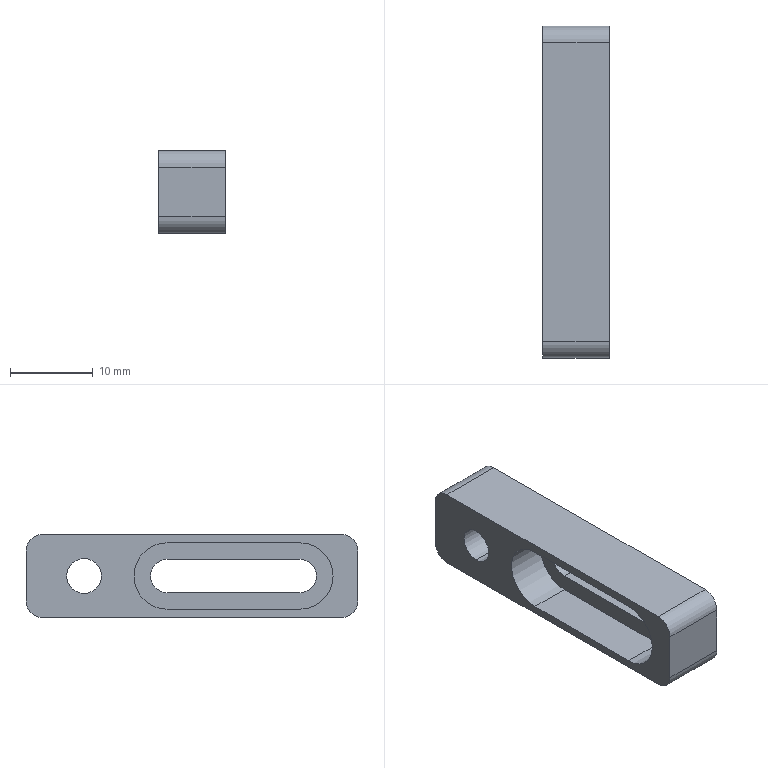Part | SolidWorks | features Fillet 2, ICE 2, Extrusion 1, HoleWzd 1 | 1 solid | 23 faces | box 8 x 40 x 10 mm | volume 1941 mm3 | cylinder 12 | plane 11 | commonest cylinder face diameters 4 x7 8 x3 4.2 x2
STEP:
#1=CARTESIAN_POINT('',(-4.756,11.524,5.));
#2=VERTEX_POINT('',#1);
#3=CARTESIAN_POINT('',(-4.756,15.524,9.));
#4=VERTEX_POINT('',#3);
#5=CARTESIAN_POINT('',(-4.756,15.524,5.));
#6=DIRECTION('',(-1.,0.,0.));
#7=DIRECTION('',(0.,-1.,0.));
#8=AXIS2_PLACEMENT_3D('',#5,#6,#7);
#9=CIRCLE('',#8,4.);
#10=EDGE_CURVE('',#2,#4,#9,.T.);
#11=ORIENTED_EDGE('',*,*,#10,.F.);
#12=CARTESIAN_POINT('',(-9.756,11.524,5.));
#13=VERTEX_POINT('',#12);
#14=CARTESIAN_POINT('',(-4.756,11.524,5.));
#15=DIRECTION('',(-1.,0.,0.));
#16=VECTOR('',#15,1000.);
#17=LINE('',#14,#16);
#18=EDGE_CURVE('',#2,#13,#17,.T.);
#19=ORIENTED_EDGE('',*,*,#18,.T.);
#20=CARTESIAN_POINT('',(-9.756,15.524,9.));
#21=VERTEX_POINT('',#20);
#22=CARTESIAN_POINT('',(-9.756,15.524,5.));
#23=DIRECTION('',(-1.,0.,0.));
#24=DIRECTION('',(0.,-1.,0.));
#25=AXIS2_PLACEMENT_3D('',#22,#23,#24);
#26=CIRCLE('',#25,4.);
#27=EDGE_CURVE('',#13,#21,#26,.T.);
#28=ORIENTED_EDGE('',*,*,#27,.T.);
#29=CARTESIAN_POINT('',(-4.756,15.524,9.));
#30=DIRECTION('',(-1.,0.,0.));
#31=VECTOR('',#30,1000.);
#32=LINE('',#29,#31);
#33=EDGE_CURVE('',#4,#21,#32,.T.);
#34=ORIENTED_EDGE('',*,*,#33,.F.);
#35=EDGE_LOOP('',(#11,#19,#28,#34));
#36=FACE_OUTER_BOUND('',#35,.T.);
#37=CARTESIAN_POINT('',(-4.756,15.524,5.));
#38=DIRECTION('',(-1.,0.,0.));
#39=DIRECTION('',(0.,-1.,0.));
#40=AXIS2_PLACEMENT_3D('',#37,#38,#39);
#41=CYLINDRICAL_SURFACE('',#40,4.);
#42=ADVANCED_FACE('',(#36),#41,.F.);
#43=CARTESIAN_POINT('',(-9.756,41.524,7.1));
#44=VERTEX_POINT('',#43);
#45=CARTESIAN_POINT('',(-9.756,41.524,2.9));
#46=VERTEX_POINT('',#45);
#47=CARTESIAN_POINT('',(-9.756,41.524,5.));
#48=DIRECTION('',(1.,0.,0.));
#49=DIRECTION('',(0.,1.,0.));
#50=AXIS2_PLACEMENT_3D('',#47,#48,#49);
#51=CIRCLE('',#50,2.1);
#52=EDGE_CURVE('',#44,#46,#51,.T.);
#53=ORIENTED_EDGE('',*,*,#52,.F.);
#54=CARTESIAN_POINT('',(-1.756,41.524,7.1));
#55=VERTEX_POINT('',#54);
#56=CARTESIAN_POINT('',(-1.756,41.524,7.1));
#57=DIRECTION('',(1.,0.,0.));
#58=VECTOR('',#57,1000.);
#59=LINE('',#56,#58);
#60=EDGE_CURVE('',#44,#55,#59,.T.);
#61=ORIENTED_EDGE('',*,*,#60,.T.);
#62=CARTESIAN_POINT('',(-1.756,41.524,2.9));
#63=VERTEX_POINT('',#62);
#64=CARTESIAN_POINT('',(-1.756,41.524,5.));
#65=DIRECTION('',(1.,0.,0.));
#66=DIRECTION('',(0.,0.,-1.));
#67=AXIS2_PLACEMENT_3D('',#64,#65,#66);
#68=CIRCLE('',#67,2.1);
#69=EDGE_CURVE('',#55,#63,#68,.T.);
#70=ORIENTED_EDGE('',*,*,#69,.T.);
#71=CARTESIAN_POINT('',(-1.756,41.524,2.9));
#72=DIRECTION('',(1.,0.,0.));
#73=VECTOR('',#72,1000.);
#74=LINE('',#71,#73);
#75=EDGE_CURVE('',#46,#63,#74,.T.);
#76=ORIENTED_EDGE('',*,*,#75,.F.);
#77=EDGE_LOOP('',(#53,#61,#70,#76));
#78=FACE_OUTER_BOUND('',#77,.T.);
#79=CARTESIAN_POINT('',(-1.756,41.524,5.));
#80=DIRECTION('',(1.,0.,0.));
#81=DIRECTION('',(0.,0.,-1.));
#82=AXIS2_PLACEMENT_3D('',#79,#80,#81);
#83=CYLINDRICAL_SURFACE('',#82,2.1);
#84=ADVANCED_FACE('',(#78),#83,.F.);
#85=CARTESIAN_POINT('',(-1.756,13.524,5.));
#86=VERTEX_POINT('',#85);
#87=CARTESIAN_POINT('',(-1.756,15.524,7.));
#88=VERTEX_POINT('',#87);
#89=CARTESIAN_POINT('',(-1.756,15.524,5.));
#90=DIRECTION('',(-1.,0.,0.));
#91=DIRECTION('',(0.,-1.,0.));
#92=AXIS2_PLACEMENT_3D('',#89,#90,#91);
#93=CIRCLE('',#92,2.);
#94=EDGE_CURVE('',#86,#88,#93,.T.);
#95=ORIENTED_EDGE('',*,*,#94,.F.);
#96=CARTESIAN_POINT('',(-4.756,13.524,5.));
#97=VERTEX_POINT('',#96);
#98=CARTESIAN_POINT('',(-1.756,13.524,5.));
#99=DIRECTION('',(-1.,0.,0.));
#100=VECTOR('',#99,1000.);
#101=LINE('',#98,#100);
#102=EDGE_CURVE('',#86,#97,#101,.T.);
#103=ORIENTED_EDGE('',*,*,#102,.T.);
#104=CARTESIAN_POINT('',(-4.756,15.524,7.));
#105=VERTEX_POINT('',#104);
#106=CARTESIAN_POINT('',(-4.756,15.524,5.));
#107=DIRECTION('',(1.,0.,0.));
#108=DIRECTION('',(0.,-1.,0.));
#109=AXIS2_PLACEMENT_3D('',#106,#107,#108);
#110=CIRCLE('',#109,2.);
#111=EDGE_CURVE('',#105,#97,#110,.T.);
#112=ORIENTED_EDGE('',*,*,#111,.F.);
#113=CARTESIAN_POINT('',(-1.756,15.524,7.));
#114=DIRECTION('',(-1.,0.,0.));
#115=VECTOR('',#114,1000.);
#116=LINE('',#113,#115);
#117=EDGE_CURVE('',#88,#105,#116,.T.);
#118=ORIENTED_EDGE('',*,*,#117,.F.);
#119=EDGE_LOOP('',(#95,#103,#112,#118));
#120=FACE_OUTER_BOUND('',#119,.T.);
#121=CARTESIAN_POINT('',(-1.756,15.524,5.));
#122=DIRECTION('',(-1.,0.,0.));
#123=DIRECTION('',(0.,-1.,0.));
#124=AXIS2_PLACEMENT_3D('',#121,#122,#123);
#125=CYLINDRICAL_SURFACE('',#124,2.);
#126=ADVANCED_FACE('',(#120),#125,.F.);
#127=ORIENTED_EDGE('',*,*,#102,.F.);
#128=CARTESIAN_POINT('',(-1.756,15.524,3.));
#129=VERTEX_POINT('',#128);
#130=CARTESIAN_POINT('',(-1.756,15.524,5.));
#131=DIRECTION('',(-1.,0.,0.));
#132=DIRECTION('',(0.,-1.,0.));
#133=AXIS2_PLACEMENT_3D('',#130,#131,#132);
#134=CIRCLE('',#133,2.);
#135=EDGE_CURVE('',#129,#86,#134,.T.);
#136=ORIENTED_EDGE('',*,*,#135,.F.);
#137=CARTESIAN_POINT('',(-4.756,15.524,3.));
#138=VERTEX_POINT('',#137);
#139=CARTESIAN_POINT('',(-1.756,15.524,3.));
#140=DIRECTION('',(-1.,0.,0.));
#141=VECTOR('',#140,1000.);
#142=LINE('',#139,#141);
#143=EDGE_CURVE('',#129,#138,#142,.T.);
#144=ORIENTED_EDGE('',*,*,#143,.T.);
#145=CARTESIAN_POINT('',(-4.756,15.524,5.));
#146=DIRECTION('',(1.,0.,0.));
#147=DIRECTION('',(0.,-1.,0.));
#148=AXIS2_PLACEMENT_3D('',#145,#146,#147);
#149=CIRCLE('',#148,2.);
#150=EDGE_CURVE('',#97,#138,#149,.T.);
#151=ORIENTED_EDGE('',*,*,#150,.F.);
#152=EDGE_LOOP('',(#127,#136,#144,#151));
#153=FACE_OUTER_BOUND('',#152,.T.);
#154=CARTESIAN_POINT('',(-1.756,15.524,5.));
#155=DIRECTION('',(-1.,0.,0.));
#156=DIRECTION('',(0.,-1.,0.));
#157=AXIS2_PLACEMENT_3D('',#154,#155,#156);
#158=CYLINDRICAL_SURFACE('',#157,2.);
#159=ADVANCED_FACE('',(#153),#158,.F.);
#160=CARTESIAN_POINT('',(-4.756,31.524,3.));
#161=VERTEX_POINT('',#160);
#162=CARTESIAN_POINT('',(-4.756,15.524,3.));
#163=DIRECTION('',(0.,1.,0.));
#164=VECTOR('',#163,1000.);
#165=LINE('',#162,#164);
#166=EDGE_CURVE('',#138,#161,#165,.T.);
#167=ORIENTED_EDGE('',*,*,#166,.F.);
#168=ORIENTED_EDGE('',*,*,#143,.F.);
#169=CARTESIAN_POINT('',(-1.756,31.524,3.));
#170=VERTEX_POINT('',#169);
#171=CARTESIAN_POINT('',(-1.756,15.524,3.));
#172=DIRECTION('',(0.,-1.,0.));
#173=VECTOR('',#172,1000.);
#174=LINE('',#171,#173);
#175=EDGE_CURVE('',#170,#129,#174,.T.);
#176=ORIENTED_EDGE('',*,*,#175,.F.);
#177=CARTESIAN_POINT('',(-1.756,31.524,3.));
#178=DIRECTION('',(-1.,0.,0.));
#179=VECTOR('',#178,1000.);
#180=LINE('',#177,#179);
#181=EDGE_CURVE('',#170,#161,#180,.T.);
#182=ORIENTED_EDGE('',*,*,#181,.T.);
#183=EDGE_LOOP('',(#167,#168,#176,#182));
#184=FACE_OUTER_BOUND('',#183,.T.);
#185=CARTESIAN_POINT('',(-1.756,15.524,3.));
#186=DIRECTION('',(0.,0.,-1.));
#187=DIRECTION('',(-1.,0.,0.));
#188=AXIS2_PLACEMENT_3D('',#185,#186,#187);
#189=PLANE('',#188);
#190=ADVANCED_FACE('',(#184),#189,.F.);
#191=CARTESIAN_POINT('',(-4.756,31.524,7.));
#192=VERTEX_POINT('',#191);
#193=CARTESIAN_POINT('',(-4.756,31.524,5.));
#194=DIRECTION('',(1.,0.,0.));
#195=DIRECTION('',(0.,-1.,0.));
#196=AXIS2_PLACEMENT_3D('',#193,#194,#195);
#197=CIRCLE('',#196,2.);
#198=EDGE_CURVE('',#161,#192,#197,.T.);
#199=ORIENTED_EDGE('',*,*,#198,.F.);
#200=ORIENTED_EDGE('',*,*,#181,.F.);
#201=CARTESIAN_POINT('',(-1.756,31.524,7.));
#202=VERTEX_POINT('',#201);
#203=CARTESIAN_POINT('',(-1.756,31.524,5.));
#204=DIRECTION('',(-1.,0.,0.));
#205=DIRECTION('',(0.,-1.,0.));
#206=AXIS2_PLACEMENT_3D('',#203,#204,#205);
#207=CIRCLE('',#206,2.);
#208=EDGE_CURVE('',#202,#170,#207,.T.);
#209=ORIENTED_EDGE('',*,*,#208,.F.);
#210=CARTESIAN_POINT('',(-1.756,31.524,7.));
#211=DIRECTION('',(-1.,0.,0.));
#212=VECTOR('',#211,1000.);
#213=LINE('',#210,#212);
#214=EDGE_CURVE('',#202,#192,#213,.T.);
#215=ORIENTED_EDGE('',*,*,#214,.T.);
#216=EDGE_LOOP('',(#199,#200,#209,#215));
#217=FACE_OUTER_BOUND('',#216,.T.);
#218=CARTESIAN_POINT('',(-1.756,31.524,5.));
#219=DIRECTION('',(-1.,0.,0.));
#220=DIRECTION('',(0.,-1.,0.));
#221=AXIS2_PLACEMENT_3D('',#218,#219,#220);
#222=CYLINDRICAL_SURFACE('',#221,2.);
#223=ADVANCED_FACE('',(#217),#222,.F.);
#224=CARTESIAN_POINT('',(-4.756,15.524,7.));
#225=DIRECTION('',(0.,-1.,0.));
#226=VECTOR('',#225,1000.);
#227=LINE('',#224,#226);
#228=EDGE_CURVE('',#192,#105,#227,.T.);
#229=ORIENTED_EDGE('',*,*,#228,.F.);
#230=ORIENTED_EDGE('',*,*,#214,.F.);
#231=CARTESIAN_POINT('',(-1.756,15.524,7.));
#232=DIRECTION('',(0.,1.,0.));
#233=VECTOR('',#232,1000.);
#234=LINE('',#231,#233);
#235=EDGE_CURVE('',#88,#202,#234,.T.);
#236=ORIENTED_EDGE('',*,*,#235,.F.);
#237=ORIENTED_EDGE('',*,*,#117,.T.);
#238=EDGE_LOOP('',(#229,#230,#236,#237));
#239=FACE_OUTER_BOUND('',#238,.T.);
#240=CARTESIAN_POINT('',(-1.756,15.524,7.));
#241=DIRECTION('',(0.,0.,1.));
#242=DIRECTION('',(1.,0.,0.));
#243=AXIS2_PLACEMENT_3D('',#240,#241,#242);
#244=PLANE('',#243);
#245=ADVANCED_FACE('',(#239),#244,.F.);
#246=CARTESIAN_POINT('',(-9.756,8.524,8.));
#247=VERTEX_POINT('',#246);
#248=CARTESIAN_POINT('',(-9.756,8.524,2.));
#249=VERTEX_POINT('',#248);
#250=CARTESIAN_POINT('',(-9.756,8.524,10.));
#251=DIRECTION('',(0.,0.,-1.));
#252=VECTOR('',#251,1000.);
#253=LINE('',#250,#252);
#254=EDGE_CURVE('',#247,#249,#253,.T.);
#255=ORIENTED_EDGE('',*,*,#254,.T.);
#256=CARTESIAN_POINT('',(-1.756,8.524,2.));
#257=VERTEX_POINT('',#256);
#258=CARTESIAN_POINT('',(-1.756,8.524,2.));
#259=DIRECTION('',(1.,0.,0.));
#260=VECTOR('',#259,1000.);
#261=LINE('',#258,#260);
#262=EDGE_CURVE('',#249,#257,#261,.T.);
#263=ORIENTED_EDGE('',*,*,#262,.T.);
#264=CARTESIAN_POINT('',(-1.756,8.524,8.));
#265=VERTEX_POINT('',#264);
#266=CARTESIAN_POINT('',(-1.756,8.524,10.));
#267=DIRECTION('',(0.,0.,-1.));
#268=VECTOR('',#267,1000.);
#269=LINE('',#266,#268);
#270=EDGE_CURVE('',#265,#257,#269,.T.);
#271=ORIENTED_EDGE('',*,*,#270,.F.);
#272=CARTESIAN_POINT('',(-9.756,8.524,8.));
#273=DIRECTION('',(-1.,0.,0.));
#274=VECTOR('',#273,1000.);
#275=LINE('',#272,#274);
#276=EDGE_CURVE('',#265,#247,#275,.T.);
#277=ORIENTED_EDGE('',*,*,#276,.T.);
#278=EDGE_LOOP('',(#255,#263,#271,#277));
#279=FACE_OUTER_BOUND('',#278,.T.);
#280=CARTESIAN_POINT('',(-1.756,8.524,10.));
#281=DIRECTION('',(0.,1.,0.));
#282=DIRECTION('',(-1.,0.,0.));
#283=AXIS2_PLACEMENT_3D('',#280,#281,#282);
#284=PLANE('',#283);
#285=ADVANCED_FACE('',(#279),#284,.F.);
#286=ORIENTED_EDGE('',*,*,#175,.T.);
#287=ORIENTED_EDGE('',*,*,#135,.T.);
#288=ORIENTED_EDGE('',*,*,#94,.T.);
#289=ORIENTED_EDGE('',*,*,#235,.T.);
#290=ORIENTED_EDGE('',*,*,#208,.T.);
#291=EDGE_LOOP('',(#286,#287,#288,#289,#290));
#292=FACE_BOUND('',#291,.T.);
#293=CARTESIAN_POINT('',(-1.756,41.524,5.));
#294=DIRECTION('',(1.,0.,0.));
#295=DIRECTION('',(0.,0.,-1.));
#296=AXIS2_PLACEMENT_3D('',#293,#294,#295);
#297=CIRCLE('',#296,2.1);
#298=EDGE_CURVE('',#63,#55,#297,.T.);
#299=ORIENTED_EDGE('',*,*,#298,.F.);
#300=ORIENTED_EDGE('',*,*,#69,.F.);
#301=EDGE_LOOP('',(#299,#300));
#302=FACE_BOUND('',#301,.T.);
#303=ORIENTED_EDGE('',*,*,#270,.T.);
#304=CARTESIAN_POINT('',(-1.756,10.524,0.));
#305=VERTEX_POINT('',#304);
#306=CARTESIAN_POINT('',(-1.756,10.524,2.));
#307=DIRECTION('',(1.,0.,0.));
#308=DIRECTION('',(0.,-1.,0.));
#309=AXIS2_PLACEMENT_3D('',#306,#307,#308);
#310=CIRCLE('',#309,2.);
#311=EDGE_CURVE('',#257,#305,#310,.T.);
#312=ORIENTED_EDGE('',*,*,#311,.T.);
#313=CARTESIAN_POINT('',(-1.756,46.524,0.));
#314=VERTEX_POINT('',#313);
#315=CARTESIAN_POINT('',(-1.756,48.524,0.));
#316=DIRECTION('',(0.,1.,0.));
#317=VECTOR('',#316,1000.);
#318=LINE('',#315,#317);
#319=EDGE_CURVE('',#305,#314,#318,.T.);
#320=ORIENTED_EDGE('',*,*,#319,.T.);
#321=CARTESIAN_POINT('',(-1.756,48.524,2.));
#322=VERTEX_POINT('',#321);
#323=CARTESIAN_POINT('',(-1.756,46.524,2.));
#324=DIRECTION('',(1.,0.,0.));
#325=DIRECTION('',(0.,-1.,0.));
#326=AXIS2_PLACEMENT_3D('',#323,#324,#325);
#327=CIRCLE('',#326,2.);
#328=EDGE_CURVE('',#314,#322,#327,.T.);
#329=ORIENTED_EDGE('',*,*,#328,.T.);
#330=CARTESIAN_POINT('',(-1.756,48.524,8.));
#331=VERTEX_POINT('',#330);
#332=CARTESIAN_POINT('',(-1.756,48.524,10.));
#333=DIRECTION('',(0.,0.,-1.));
#334=VECTOR('',#333,1000.);
#335=LINE('',#332,#334);
#336=EDGE_CURVE('',#331,#322,#335,.T.);
#337=ORIENTED_EDGE('',*,*,#336,.F.);
#338=CARTESIAN_POINT('',(-1.756,46.524,10.));
#339=VERTEX_POINT('',#338);
#340=CARTESIAN_POINT('',(-1.756,46.524,8.));
#341=DIRECTION('',(1.,0.,0.));
#342=DIRECTION('',(0.,-1.,0.));
#343=AXIS2_PLACEMENT_3D('',#340,#341,#342);
#344=CIRCLE('',#343,2.);
#345=EDGE_CURVE('',#331,#339,#344,.T.);
#346=ORIENTED_EDGE('',*,*,#345,.T.);
#347=CARTESIAN_POINT('',(-1.756,10.524,10.));
#348=VERTEX_POINT('',#347);
#349=CARTESIAN_POINT('',(-1.756,48.524,10.));
#350=DIRECTION('',(0.,1.,0.));
#351=VECTOR('',#350,1000.);
#352=LINE('',#349,#351);
#353=EDGE_CURVE('',#348,#339,#352,.T.);
#354=ORIENTED_EDGE('',*,*,#353,.F.);
#355=CARTESIAN_POINT('',(-1.756,10.524,8.));
#356=DIRECTION('',(1.,0.,0.));
#357=DIRECTION('',(0.,-1.,0.));
#358=AXIS2_PLACEMENT_3D('',#355,#356,#357);
#359=CIRCLE('',#358,2.);
#360=EDGE_CURVE('',#348,#265,#359,.T.);
#361=ORIENTED_EDGE('',*,*,#360,.T.);
#362=EDGE_LOOP('',(#303,#312,#320,#329,#337,#346,#354,#361));
#363=FACE_OUTER_BOUND('',#362,.T.);
#364=CARTESIAN_POINT('',(-1.756,48.524,10.));
#365=DIRECTION('',(-1.,0.,0.));
#366=DIRECTION('',(0.,-1.,0.));
#367=AXIS2_PLACEMENT_3D('',#364,#365,#366);
#368=PLANE('',#367);
#369=ADVANCED_FACE('',(#292,#302,#363),#368,.F.);
#370=ORIENTED_EDGE('',*,*,#336,.T.);
#371=CARTESIAN_POINT('',(-9.756,48.524,2.));
#372=VERTEX_POINT('',#371);
#373=CARTESIAN_POINT('',(-9.756,48.524,2.));
#374=DIRECTION('',(-1.,0.,0.));
#375=VECTOR('',#374,1000.);
#376=LINE('',#373,#375);
#377=EDGE_CURVE('',#322,#372,#376,.T.);
#378=ORIENTED_EDGE('',*,*,#377,.T.);
#379=CARTESIAN_POINT('',(-9.756,48.524,8.));
#380=VERTEX_POINT('',#379);
#381=CARTESIAN_POINT('',(-9.756,48.524,10.));
#382=DIRECTION('',(0.,0.,-1.));
#383=VECTOR('',#382,1000.);
#384=LINE('',#381,#383);
#385=EDGE_CURVE('',#380,#372,#384,.T.);
#386=ORIENTED_EDGE('',*,*,#385,.F.);
#387=CARTESIAN_POINT('',(-1.756,48.524,8.));
#388=DIRECTION('',(1.,0.,0.));
#389=VECTOR('',#388,1000.);
#390=LINE('',#387,#389);
#391=EDGE_CURVE('',#380,#331,#390,.T.);
#392=ORIENTED_EDGE('',*,*,#391,.T.);
#393=EDGE_LOOP('',(#370,#378,#386,#392));
#394=FACE_OUTER_BOUND('',#393,.T.);
#395=CARTESIAN_POINT('',(-9.756,48.524,10.));
#396=DIRECTION('',(0.,-1.,0.));
#397=DIRECTION('',(0.,0.,-1.));
#398=AXIS2_PLACEMENT_3D('',#395,#396,#397);
#399=PLANE('',#398);
#400=ADVANCED_FACE('',(#394),#399,.F.);
#401=CARTESIAN_POINT('',(-9.756,31.524,1.));
#402=VERTEX_POINT('',#401);
#403=CARTESIAN_POINT('',(-9.756,15.524,1.));
#404=VERTEX_POINT('',#403);
#405=CARTESIAN_POINT('',(-9.756,31.524,1.));
#406=DIRECTION('',(0.,-1.,0.));
#407=VECTOR('',#406,1000.);
#408=LINE('',#405,#407);
#409=EDGE_CURVE('',#402,#404,#408,.T.);
#410=ORIENTED_EDGE('',*,*,#409,.F.);
#411=CARTESIAN_POINT('',(-9.756,31.524,9.));
#412=VERTEX_POINT('',#411);
#413=CARTESIAN_POINT('',(-9.756,31.524,5.));
#414=DIRECTION('',(-1.,0.,0.));
#415=DIRECTION('',(0.,-1.,0.));
#416=AXIS2_PLACEMENT_3D('',#413,#414,#415);
#417=CIRCLE('',#416,4.);
#418=EDGE_CURVE('',#412,#402,#417,.T.);
#419=ORIENTED_EDGE('',*,*,#418,.F.);
#420=CARTESIAN_POINT('',(-9.756,31.524,9.));
#421=DIRECTION('',(0.,1.,0.));
#422=VECTOR('',#421,1000.);
#423=LINE('',#420,#422);
#424=EDGE_CURVE('',#21,#412,#423,.T.);
#425=ORIENTED_EDGE('',*,*,#424,.F.);
#426=ORIENTED_EDGE('',*,*,#27,.F.);
#427=CARTESIAN_POINT('',(-9.756,15.524,5.));
#428=DIRECTION('',(-1.,0.,0.));
#429=DIRECTION('',(0.,-1.,0.));
#430=AXIS2_PLACEMENT_3D('',#427,#428,#429);
#431=CIRCLE('',#430,4.);
#432=EDGE_CURVE('',#404,#13,#431,.T.);
#433=ORIENTED_EDGE('',*,*,#432,.F.);
#434=EDGE_LOOP('',(#410,#419,#425,#426,#433));
#435=FACE_BOUND('',#434,.T.);
#436=CARTESIAN_POINT('',(-9.756,41.524,5.));
#437=DIRECTION('',(1.,0.,0.));
#438=DIRECTION('',(0.,1.,0.));
#439=AXIS2_PLACEMENT_3D('',#436,#437,#438);
#440=CIRCLE('',#439,2.1);
#441=EDGE_CURVE('',#46,#44,#440,.T.);
#442=ORIENTED_EDGE('',*,*,#441,.T.);
#443=ORIENTED_EDGE('',*,*,#52,.T.);
#444=EDGE_LOOP('',(#442,#443));
#445=FACE_BOUND('',#444,.T.);
#446=CARTESIAN_POINT('',(-9.756,46.524,0.));
#447=VERTEX_POINT('',#446);
#448=CARTESIAN_POINT('',(-9.756,10.524,0.));
#449=VERTEX_POINT('',#448);
#450=CARTESIAN_POINT('',(-9.756,48.524,0.));
#451=DIRECTION('',(0.,-1.,0.));
#452=VECTOR('',#451,1000.);
#453=LINE('',#450,#452);
#454=EDGE_CURVE('',#447,#449,#453,.T.);
#455=ORIENTED_EDGE('',*,*,#454,.T.);
#456=CARTESIAN_POINT('',(-9.756,10.524,2.));
#457=DIRECTION('',(-1.,0.,0.));
#458=DIRECTION('',(0.,1.,0.));
#459=AXIS2_PLACEMENT_3D('',#456,#457,#458);
#460=CIRCLE('',#459,2.);
#461=EDGE_CURVE('',#449,#249,#460,.T.);
#462=ORIENTED_EDGE('',*,*,#461,.T.);
#463=ORIENTED_EDGE('',*,*,#254,.F.);
#464=CARTESIAN_POINT('',(-9.756,10.524,10.));
#465=VERTEX_POINT('',#464);
#466=CARTESIAN_POINT('',(-9.756,10.524,8.));
#467=DIRECTION('',(-1.,0.,0.));
#468=DIRECTION('',(0.,1.,0.));
#469=AXIS2_PLACEMENT_3D('',#466,#467,#468);
#470=CIRCLE('',#469,2.);
#471=EDGE_CURVE('',#247,#465,#470,.T.);
#472=ORIENTED_EDGE('',*,*,#471,.T.);
#473=CARTESIAN_POINT('',(-9.756,46.524,10.));
#474=VERTEX_POINT('',#473);
#475=CARTESIAN_POINT('',(-9.756,48.524,10.));
#476=DIRECTION('',(0.,-1.,0.));
#477=VECTOR('',#476,1000.);
#478=LINE('',#475,#477);
#479=EDGE_CURVE('',#474,#465,#478,.T.);
#480=ORIENTED_EDGE('',*,*,#479,.F.);
#481=CARTESIAN_POINT('',(-9.756,46.524,8.));
#482=DIRECTION('',(-1.,0.,0.));
#483=DIRECTION('',(0.,1.,0.));
#484=AXIS2_PLACEMENT_3D('',#481,#482,#483);
#485=CIRCLE('',#484,2.);
#486=EDGE_CURVE('',#474,#380,#485,.T.);
#487=ORIENTED_EDGE('',*,*,#486,.T.);
#488=ORIENTED_EDGE('',*,*,#385,.T.);
#489=CARTESIAN_POINT('',(-9.756,46.524,2.));
#490=DIRECTION('',(-1.,0.,0.));
#491=DIRECTION('',(0.,1.,0.));
#492=AXIS2_PLACEMENT_3D('',#489,#490,#491);
#493=CIRCLE('',#492,2.);
#494=EDGE_CURVE('',#372,#447,#493,.T.);
#495=ORIENTED_EDGE('',*,*,#494,.T.);
#496=EDGE_LOOP('',(#455,#462,#463,#472,#480,#487,#488,#495));
#497=FACE_OUTER_BOUND('',#496,.T.);
#498=CARTESIAN_POINT('',(-9.756,48.524,10.));
#499=DIRECTION('',(1.,0.,0.));
#500=DIRECTION('',(0.,1.,0.));
#501=AXIS2_PLACEMENT_3D('',#498,#499,#500);
#502=PLANE('',#501);
#503=ADVANCED_FACE('',(#435,#445,#497),#502,.F.);
#504=ORIENTED_EDGE('',*,*,#479,.T.);
#505=CARTESIAN_POINT('',(-1.756,10.524,10.));
#506=DIRECTION('',(1.,0.,0.));
#507=VECTOR('',#506,1000.);
#508=LINE('',#505,#507);
#509=EDGE_CURVE('',#465,#348,#508,.T.);
#510=ORIENTED_EDGE('',*,*,#509,.T.);
#511=ORIENTED_EDGE('',*,*,#353,.T.);
#512=CARTESIAN_POINT('',(-9.756,46.524,10.));
#513=DIRECTION('',(-1.,0.,0.));
#514=VECTOR('',#513,1000.);
#515=LINE('',#512,#514);
#516=EDGE_CURVE('',#339,#474,#515,.T.);
#517=ORIENTED_EDGE('',*,*,#516,.T.);
#518=EDGE_LOOP('',(#504,#510,#511,#517));
#519=FACE_OUTER_BOUND('',#518,.T.);
#520=CARTESIAN_POINT('',(0.,0.,10.));
#521=DIRECTION('',(0.,0.,1.));
#522=DIRECTION('',(1.,0.,0.));
#523=AXIS2_PLACEMENT_3D('',#520,#521,#522);
#524=PLANE('',#523);
#525=ADVANCED_FACE('',(#519),#524,.T.);
#526=ORIENTED_EDGE('',*,*,#319,.F.);
#527=CARTESIAN_POINT('',(0.,10.524,0.));
#528=DIRECTION('',(-1.,0.,0.));
#529=VECTOR('',#528,1000.);
#530=LINE('',#527,#529);
#531=EDGE_CURVE('',#305,#449,#530,.T.);
#532=ORIENTED_EDGE('',*,*,#531,.T.);
#533=ORIENTED_EDGE('',*,*,#454,.F.);
#534=CARTESIAN_POINT('',(0.,46.524,0.));
#535=DIRECTION('',(1.,0.,0.));
#536=VECTOR('',#535,1000.);
#537=LINE('',#534,#536);
#538=EDGE_CURVE('',#447,#314,#537,.T.);
#539=ORIENTED_EDGE('',*,*,#538,.T.);
#540=EDGE_LOOP('',(#526,#532,#533,#539));
#541=FACE_OUTER_BOUND('',#540,.T.);
#542=CARTESIAN_POINT('',(0.,0.,0.));
#543=DIRECTION('',(0.,0.,1.));
#544=DIRECTION('',(1.,0.,0.));
#545=AXIS2_PLACEMENT_3D('',#542,#543,#544);
#546=PLANE('',#545);
#547=ADVANCED_FACE('',(#541),#546,.F.);
#548=ORIENTED_EDGE('',*,*,#60,.F.);
#549=ORIENTED_EDGE('',*,*,#441,.F.);
#550=ORIENTED_EDGE('',*,*,#75,.T.);
#551=ORIENTED_EDGE('',*,*,#298,.T.);
#552=EDGE_LOOP('',(#548,#549,#550,#551));
#553=FACE_OUTER_BOUND('',#552,.T.);
#554=CARTESIAN_POINT('',(-1.756,41.524,5.));
#555=DIRECTION('',(1.,0.,0.));
#556=DIRECTION('',(0.,0.,-1.));
#557=AXIS2_PLACEMENT_3D('',#554,#555,#556);
#558=CYLINDRICAL_SURFACE('',#557,2.1);
#559=ADVANCED_FACE('',(#553),#558,.F.);
#560=ORIENTED_EDGE('',*,*,#328,.F.);
#561=ORIENTED_EDGE('',*,*,#538,.F.);
#562=ORIENTED_EDGE('',*,*,#494,.F.);
#563=ORIENTED_EDGE('',*,*,#377,.F.);
#564=EDGE_LOOP('',(#560,#561,#562,#563));
#565=FACE_OUTER_BOUND('',#564,.T.);
#566=CARTESIAN_POINT('',(-9.756,46.524,2.));
#567=DIRECTION('',(-1.,0.,0.));
#568=DIRECTION('',(0.,0.,1.));
#569=AXIS2_PLACEMENT_3D('',#566,#567,#568);
#570=CYLINDRICAL_SURFACE('',#569,2.);
#571=ADVANCED_FACE('',(#565),#570,.T.);
#572=ORIENTED_EDGE('',*,*,#345,.F.);
#573=ORIENTED_EDGE('',*,*,#391,.F.);
#574=ORIENTED_EDGE('',*,*,#486,.F.);
#575=ORIENTED_EDGE('',*,*,#516,.F.);
#576=EDGE_LOOP('',(#572,#573,#574,#575));
#577=FACE_OUTER_BOUND('',#576,.T.);
#578=CARTESIAN_POINT('',(0.,46.524,8.));
#579=DIRECTION('',(1.,0.,0.));
#580=DIRECTION('',(0.,0.,-1.));
#581=AXIS2_PLACEMENT_3D('',#578,#579,#580);
#582=CYLINDRICAL_SURFACE('',#581,2.);
#583=ADVANCED_FACE('',(#577),#582,.T.);
#584=CARTESIAN_POINT('',(-4.756,31.524,9.));
#585=VERTEX_POINT('',#584);
#586=CARTESIAN_POINT('',(-4.756,31.524,1.));
#587=VERTEX_POINT('',#586);
#588=CARTESIAN_POINT('',(-4.756,31.524,5.));
#589=DIRECTION('',(-1.,0.,0.));
#590=DIRECTION('',(0.,-1.,0.));
#591=AXIS2_PLACEMENT_3D('',#588,#589,#590);
#592=CIRCLE('',#591,4.);
#593=EDGE_CURVE('',#585,#587,#592,.T.);
#594=ORIENTED_EDGE('',*,*,#593,.T.);
#595=CARTESIAN_POINT('',(-4.756,15.524,1.));
#596=VERTEX_POINT('',#595);
#597=CARTESIAN_POINT('',(-4.756,31.524,1.));
#598=DIRECTION('',(0.,-1.,0.));
#599=VECTOR('',#598,1000.);
#600=LINE('',#597,#599);
#601=EDGE_CURVE('',#587,#596,#600,.T.);
#602=ORIENTED_EDGE('',*,*,#601,.T.);
#603=CARTESIAN_POINT('',(-4.756,15.524,5.));
#604=DIRECTION('',(-1.,0.,0.));
#605=DIRECTION('',(0.,-1.,0.));
#606=AXIS2_PLACEMENT_3D('',#603,#604,#605);
#607=CIRCLE('',#606,4.);
#608=EDGE_CURVE('',#596,#2,#607,.T.);
#609=ORIENTED_EDGE('',*,*,#608,.T.);
#610=ORIENTED_EDGE('',*,*,#10,.T.);
#611=CARTESIAN_POINT('',(-4.756,31.524,9.));
#612=DIRECTION('',(0.,1.,0.));
#613=VECTOR('',#612,1000.);
#614=LINE('',#611,#613);
#615=EDGE_CURVE('',#4,#585,#614,.T.);
#616=ORIENTED_EDGE('',*,*,#615,.T.);
#617=EDGE_LOOP('',(#594,#602,#609,#610,#616));
#618=FACE_OUTER_BOUND('',#617,.T.);
#619=ORIENTED_EDGE('',*,*,#111,.T.);
#620=ORIENTED_EDGE('',*,*,#150,.T.);
#621=ORIENTED_EDGE('',*,*,#166,.T.);
#622=ORIENTED_EDGE('',*,*,#198,.T.);
#623=ORIENTED_EDGE('',*,*,#228,.T.);
#624=EDGE_LOOP('',(#619,#620,#621,#622,#623));
#625=FACE_BOUND('',#624,.T.);
#626=CARTESIAN_POINT('',(-4.756,31.524,5.));
#627=DIRECTION('',(-1.,0.,0.));
#628=DIRECTION('',(0.,-1.,0.));
#629=AXIS2_PLACEMENT_3D('',#626,#627,#628);
#630=PLANE('',#629);
#631=ADVANCED_FACE('',(#618,#625),#630,.T.);
#632=ORIENTED_EDGE('',*,*,#418,.T.);
#633=CARTESIAN_POINT('',(-4.756,31.524,1.));
#634=DIRECTION('',(-1.,0.,0.));
#635=VECTOR('',#634,1000.);
#636=LINE('',#633,#635);
#637=EDGE_CURVE('',#587,#402,#636,.T.);
#638=ORIENTED_EDGE('',*,*,#637,.F.);
#639=ORIENTED_EDGE('',*,*,#593,.F.);
#640=CARTESIAN_POINT('',(-4.756,31.524,9.));
#641=DIRECTION('',(-1.,0.,0.));
#642=VECTOR('',#641,1000.);
#643=LINE('',#640,#642);
#644=EDGE_CURVE('',#585,#412,#643,.T.);
#645=ORIENTED_EDGE('',*,*,#644,.T.);
#646=EDGE_LOOP('',(#632,#638,#639,#645));
#647=FACE_OUTER_BOUND('',#646,.T.);
#648=CARTESIAN_POINT('',(-4.756,31.524,5.));
#649=DIRECTION('',(-1.,0.,0.));
#650=DIRECTION('',(0.,-1.,0.));
#651=AXIS2_PLACEMENT_3D('',#648,#649,#650);
#652=CYLINDRICAL_SURFACE('',#651,4.);
#653=ADVANCED_FACE('',(#647),#652,.F.);
#654=ORIENTED_EDGE('',*,*,#424,.T.);
#655=ORIENTED_EDGE('',*,*,#644,.F.);
#656=ORIENTED_EDGE('',*,*,#615,.F.);
#657=ORIENTED_EDGE('',*,*,#33,.T.);
#658=EDGE_LOOP('',(#654,#655,#656,#657));
#659=FACE_OUTER_BOUND('',#658,.T.);
#660=CARTESIAN_POINT('',(-4.756,31.524,9.));
#661=DIRECTION('',(0.,0.,1.));
#662=DIRECTION('',(0.,-1.,0.));
#663=AXIS2_PLACEMENT_3D('',#660,#661,#662);
#664=PLANE('',#663);
#665=ADVANCED_FACE('',(#659),#664,.F.);
#666=ORIENTED_EDGE('',*,*,#18,.F.);
#667=ORIENTED_EDGE('',*,*,#608,.F.);
#668=CARTESIAN_POINT('',(-4.756,15.524,1.));
#669=DIRECTION('',(-1.,0.,0.));
#670=VECTOR('',#669,1000.);
#671=LINE('',#668,#670);
#672=EDGE_CURVE('',#596,#404,#671,.T.);
#673=ORIENTED_EDGE('',*,*,#672,.T.);
#674=ORIENTED_EDGE('',*,*,#432,.T.);
#675=EDGE_LOOP('',(#666,#667,#673,#674));
#676=FACE_OUTER_BOUND('',#675,.T.);
#677=CARTESIAN_POINT('',(-4.756,15.524,5.));
#678=DIRECTION('',(-1.,0.,0.));
#679=DIRECTION('',(0.,-1.,0.));
#680=AXIS2_PLACEMENT_3D('',#677,#678,#679);
#681=CYLINDRICAL_SURFACE('',#680,4.);
#682=ADVANCED_FACE('',(#676),#681,.F.);
#683=ORIENTED_EDGE('',*,*,#409,.T.);
#684=ORIENTED_EDGE('',*,*,#672,.F.);
#685=ORIENTED_EDGE('',*,*,#601,.F.);
#686=ORIENTED_EDGE('',*,*,#637,.T.);
#687=EDGE_LOOP('',(#683,#684,#685,#686));
#688=FACE_OUTER_BOUND('',#687,.T.);
#689=CARTESIAN_POINT('',(-4.756,31.524,1.));
#690=DIRECTION('',(0.,0.,-1.));
#691=DIRECTION('',(0.,1.,0.));
#692=AXIS2_PLACEMENT_3D('',#689,#690,#691);
#693=PLANE('',#692);
#694=ADVANCED_FACE('',(#688),#693,.F.);
#695=ORIENTED_EDGE('',*,*,#461,.F.);
#696=ORIENTED_EDGE('',*,*,#531,.F.);
#697=ORIENTED_EDGE('',*,*,#311,.F.);
#698=ORIENTED_EDGE('',*,*,#262,.F.);
#699=EDGE_LOOP('',(#695,#696,#697,#698));
#700=FACE_OUTER_BOUND('',#699,.T.);
#701=CARTESIAN_POINT('',(-1.756,10.524,2.));
#702=DIRECTION('',(1.,0.,0.));
#703=DIRECTION('',(0.,1.,0.));
#704=AXIS2_PLACEMENT_3D('',#701,#702,#703);
#705=CYLINDRICAL_SURFACE('',#704,2.);
#706=ADVANCED_FACE('',(#700),#705,.T.);
#707=ORIENTED_EDGE('',*,*,#471,.F.);
#708=ORIENTED_EDGE('',*,*,#276,.F.);
#709=ORIENTED_EDGE('',*,*,#360,.F.);
#710=ORIENTED_EDGE('',*,*,#509,.F.);
#711=EDGE_LOOP('',(#707,#708,#709,#710));
#712=FACE_OUTER_BOUND('',#711,.T.);
#713=CARTESIAN_POINT('',(0.,10.524,8.));
#714=DIRECTION('',(-1.,0.,0.));
#715=DIRECTION('',(0.,-1.,0.));
#716=AXIS2_PLACEMENT_3D('',#713,#714,#715);
#717=CYLINDRICAL_SURFACE('',#716,2.);
#718=ADVANCED_FACE('',(#712),#717,.T.);
#719=CLOSED_SHELL('',(#42,#84,#126,#159,#190,#223,#245,#285,#369,#400,#503,#525,#547,#559,#571,#583,#631,#653,#665,#682,#694,#706,#718));
#720=MANIFOLD_SOLID_BREP('',#719);
#721=CARTESIAN_POINT('',(0.,0.,0.));
#722=DIRECTION('',(0.,0.,1.));
#723=DIRECTION('',(1.,0.,0.));
#724=AXIS2_PLACEMENT_3D('',#721,#722,#723);
#725=(LENGTH_UNIT()NAMED_UNIT(*)SI_UNIT(.MILLI.,.METRE.));
#726=UNCERTAINTY_MEASURE_WITH_UNIT(LENGTH_MEASURE(0.00001),#725,'','');
#727=(NAMED_UNIT(*)PLANE_ANGLE_UNIT()SI_UNIT($,.RADIAN.));
#728=(NAMED_UNIT(*)SI_UNIT($,.STERADIAN.)SOLID_ANGLE_UNIT());
#729=(GEOMETRIC_REPRESENTATION_CONTEXT(3)GLOBAL_UNCERTAINTY_ASSIGNED_CONTEXT((#726))GLOBAL_UNIT_ASSIGNED_CONTEXT((#725,#727,#728))REPRESENTATION_CONTEXT('',''));
#730=ADVANCED_BREP_SHAPE_REPRESENTATION('',(#720,#724),#729);